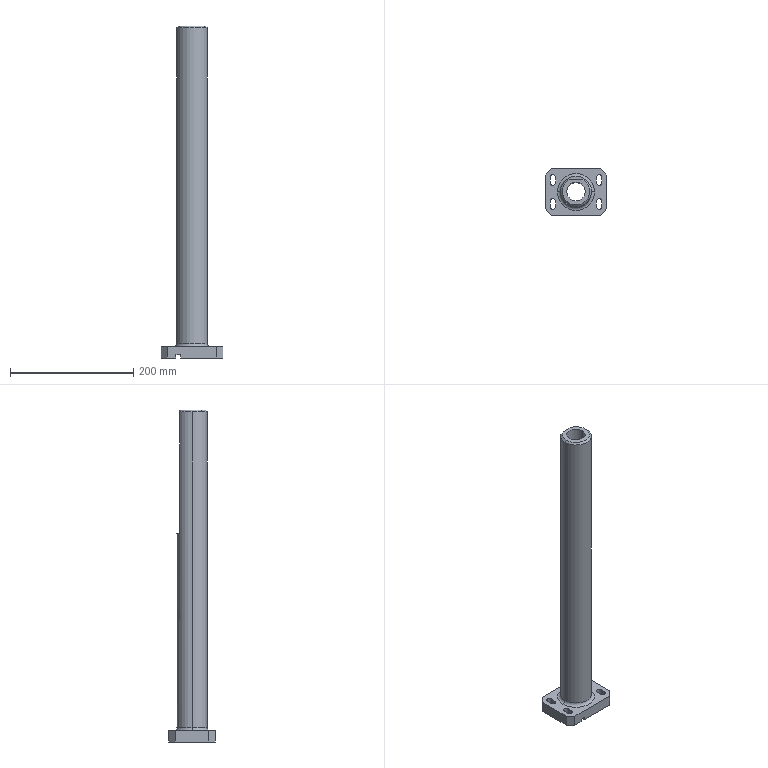Part | STEP file | PN_0008 | 1 solid | 42 faces | box 100 x 75 x 538 mm | volume 739254 mm3 | plane 25 | cylinder 12 | cone 3 | torus 2 | commonest cylinder face diameters 9 x8 30 x2 50 x2